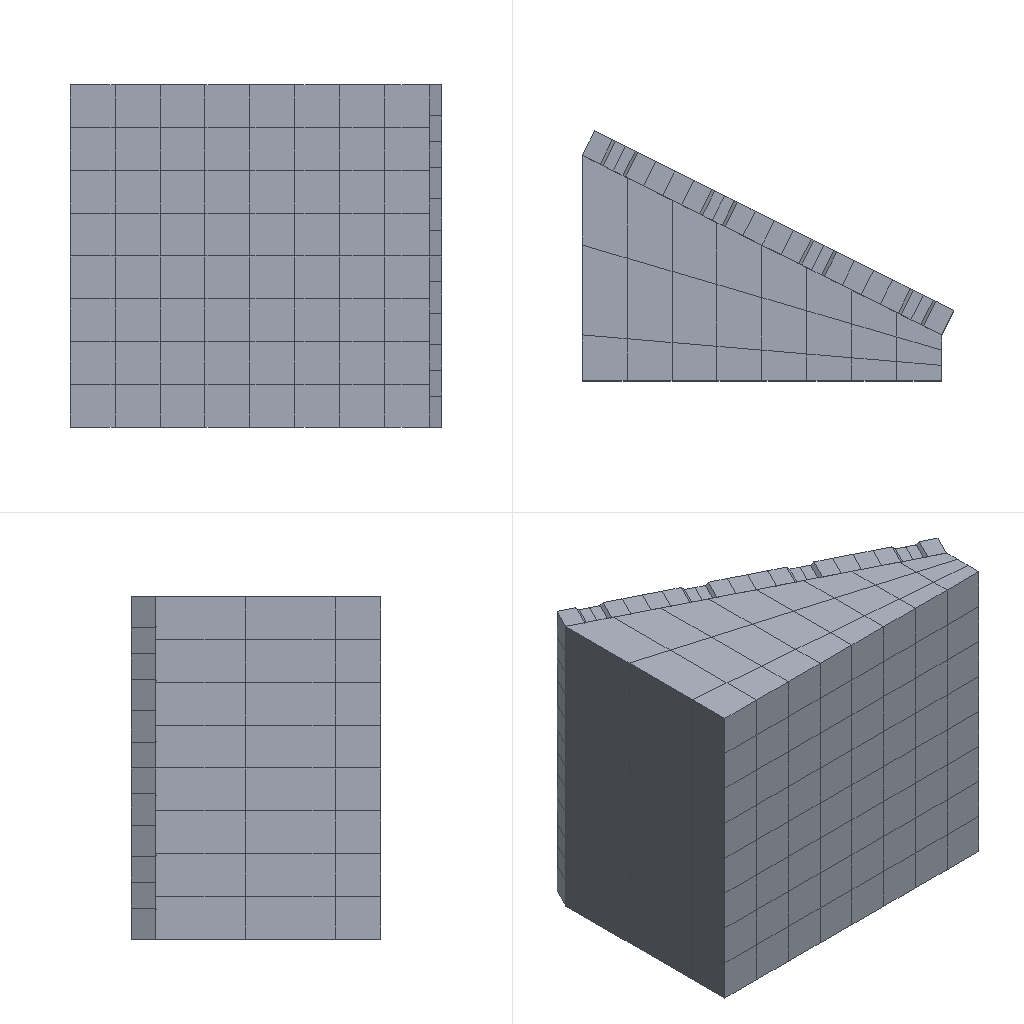Simulation study | abaqus
Set-up summary:
category,name,step,type,value,unit,region
solver,abaqus
solver,version,,,Abaqus/Standard 2020
units,not stated in the deck,,not stated
analysis,deck,,transient,transient
load_step,Step-2,Step-2,transient
load_step,requested,,,1
mesh,nodes,,,3205
mesh,elements,,,1224
element_type,C3D8R,,solid,1224
load,load commands in deck,,count,6
bc,support commands in deck,,count,8
material,HUNNINGTU,,in results
material,S,,in results
check,setup vs results,,match,"per instance, exact: element labels, types and connectivity; labels of the nodes the elements use; coordinates of those nodes at SINGLE_PRECISION in 15 of 31 instance(s)"
Abaqus input file, long lists of numbers shortened, first 402 of 1279 lines:
*Heading
** Job name: Job-1 Model name: Job-9
** Generated by: Abaqus/CAE 2020
*Preprint, echo=NO, model=NO, history=NO, contact=NO
**
** PARTS
**
*Part, name=BIKONGQIKUAI1
*Node
      1,  -23.409,         -15.,          12.
      2,  -23.409,  -10.17,          12.
** (128 more lines like these left out)
*Element, type=C3D8R
 1,  26,  33,  60,  27,  91,  98, 125,  92
 2,   1,   2,  44,  35,  66,  67, 109, 100
** (46 more lines like these left out)
*Nset, nset=SET-1, generate
   1,  130,    1
*Elset, elset=SET-1, generate
  1,  48,   1
** Section: Section-2-SET-1
*Solid Section, elset=SET-1, material=HUNNINGTU
,
*End Part
**
*Part, name=BIKONGQIKUAI1-COPY
*Node
      1,  0.1705,  -24.319,           0.
      2,  0.1705,  -5.681,           0.
** (62 more lines like these left out)
*Element, type=C3D8R
 1, 21,  3, 29, 25, 53, 35, 61, 57
 2, 22, 32, 30, 20, 54, 64, 62, 52
** (20 more lines like these left out)
*Nset, nset=SET-1, generate
  1,  64,   1
*Elset, elset=SET-1, generate
  1,  22,   1
** Section: Section-3-SET-1
*Solid Section, elset=SET-1, material=HUNNINGTU
,
*End Part
**
*Part, name=BIKONGQIKUAI1-COPY2
*Node
      1,   13.807,  -3.411,          12.
      2,   13.807,  -5.681,          12.
** (24 more lines like these left out)
*Element, type=C3D8R
1,  5, 18,  2,  1,  8, 24, 12, 13
2, 20,  3, 18,  5, 21, 23, 24,  8
** (4 more lines like these left out)
*Nset, nset=TIANCHONG, generate
  1,  26,   1
*Elset, elset=TIANCHONG, generate
 1,  6,  1
** Section: Section-4-TIANCHONG
*Solid Section, elset=TIANCHONG, material=HUNNINGTU
,
*End Part
**
*Part, name=PART-6
*Node
      1,  -157.419,   78.696,         150.
      2,  -137.741,   68.859,         150.
** (323 more lines like these left out)
*Element, type=C3D8R
  1,  82,  83,  92,  91,   1,   2,  11,  10
  2,  83,  84,  93,  92,   2,   3,  12,  11
** (190 more lines like these left out)
*Nset, nset=PART-6-REFPT_, internal
 325,
*Nset, nset=SET-2, generate
   1,  324,    1
*Elset, elset=SET-2, generate
   1,  192,    1
** Section: Section-1-SET-2
*Solid Section, elset=SET-2, material=S
,
*End Part
**
**
** ASSEMBLY
**
*Assembly, name=Assembly
**
*Instance, name=PART-6-1, part=PART-6
*End Instance
**
*Instance, name=BIKONGQIKUAI1-1, part=BIKONGQIKUAI1
-26.827, 13.414, 125.171
-26.827, 13.414, 125.171, -27.292, 14.167, 125.636, 106.047
*End Instance
**
*Instance, name=BIKONGQIKUAI1-COPY-1, part=BIKONGQIKUAI1-COPY
-48.579, 24.288, 150.171
-48.579, 24.288, 150.171, -49.045, 25.041, 150.636, 106.047
*End Instance
**
*Instance, name=BIKONGQIKUAI1-COPY2-1, part=BIKONGQIKUAI1-COPY2
-5.359, -10.734, 124.83
-5.359, -10.734, 124.83, -4.711, -10.333, 125.477, 223.65
*End Instance
**
*Instance, name=BIKONGQIKUAI1-1-LIN-1-2, part=BIKONGQIKUAI1
-26.827, 13.414, 75.171
-26.827, 13.414, 75.171, -27.292, 14.167, 75.636, 106.047
*End Instance
**
*Instance, name=BIKONGQIKUAI1-1-LIN-1-3, part=BIKONGQIKUAI1
-26.827, 13.414, 25.171
-26.827, 13.414, 25.171, -27.292, 14.167, 25.636, 106.047
*End Instance
**
*Instance, name=BIKONGQIKUAI1-1-LIN-2-1, part=BIKONGQIKUAI1
-48.579, 24.288, 100.17
-48.579, 24.288, 100.17, -49.045, 25.041, 100.635, 106.047
*End Instance
**
*Instance, name=BIKONGQIKUAI1-1-LIN-2-2, part=BIKONGQIKUAI1
-48.579, 24.288, 50.171
-48.579, 24.288, 50.171, -49.045, 25.041, 50.636, 106.047
*End Instance
**
*Instance, name=BIKONGQIKUAI1-1-LIN-2-3, part=BIKONGQIKUAI1
-70.331, 35.161, 25.17
-70.331, 35.161, 25.17, -70.797, 35.914, 25.635, 106.047
*End Instance
**
*Instance, name=BIKONGQIKUAI1-1-LIN-3-1, part=BIKONGQIKUAI1
-113.835, 56.909, 125.172
-113.835, 56.909, 125.172, -114.301, 57.662, 125.637, 106.047
*End Instance
**
*Instance, name=BIKONGQIKUAI1-1-LIN-3-2, part=BIKONGQIKUAI1
-92.083, 46.035, 100.171
-92.083, 46.035, 100.171, -92.549, 46.788, 100.636, 106.047
*End Instance
**
*Instance, name=BIKONGQIKUAI1-1-LIN-3-3, part=BIKONGQIKUAI1
-92.083, 46.035, 50.171
-92.083, 46.035, 50.171, -92.549, 46.788, 50.636, 106.047
*End Instance
**
*Instance, name=BIKONGQIKUAI1-1-LIN-4-1, part=BIKONGQIKUAI1
-113.835, 56.909, 75.17
-113.835, 56.909, 75.17, -114.301, 57.662, 75.635, 106.047
*End Instance
**
*Instance, name=BIKONGQIKUAI1-1-LIN-4-2, part=BIKONGQIKUAI1
-135.587, 67.782, 100.171
-135.587, 67.782, 100.171, -136.053, 68.535, 100.636, 106.047
*End Instance
**
*Instance, name=BIKONGQIKUAI1-1-LIN-4-3, part=BIKONGQIKUAI1
-157.34, 78.656, 125.172
-157.34, 78.656, 125.172, -157.805, 79.409, 125.637, 106.047
*End Instance
**
*Instance, name=BIKONGQIKUAI1-1-LIN-2-3-LIN-2-1, part=BIKONGQIKUAI1
-70.331, 35.161, 75.17
-70.331, 35.161, 75.17, -70.797, 35.914, 75.635, 106.047
*End Instance
**
*Instance, name=BIKONGQIKUAI1-1-LIN-2-3-LIN-3-1, part=BIKONGQIKUAI1
-70.331, 35.161, 125.17
-70.331, 35.161, 125.17, -70.797, 35.914, 125.635, 106.047
*End Instance
**
*Instance, name=BIKONGQIKUAI1-1-LIN-4-3-LIN-2-1, part=BIKONGQIKUAI1
-157.34, 78.656, 75.172
-157.34, 78.656, 75.172, -157.805, 79.409, 75.637, 106.047
*End Instance
**
*Instance, name=BIKONGQIKUAI1-1-LIN-4-3-LIN-3-1, part=BIKONGQIKUAI1
-157.34, 78.656, 25.172
-157.34, 78.656, 25.172, -157.805, 79.409, 25.637, 106.047
*End Instance
**
*Instance, name=BIKONGQIKUAI1-1-LIN-4-2-LIN-2-1, part=BIKONGQIKUAI1
-135.587, 67.782, 50.171
-135.587, 67.782, 50.171, -136.053, 68.535, 50.636, 106.047
*End Instance
**
*Instance, name=BIKONGQIKUAI1-1-LIN-4-2-LIN-3-1, part=BIKONGQIKUAI1
-113.835, 56.909, 25.17
-113.835, 56.909, 25.17, -114.301, 57.662, 25.635, 106.047
*End Instance
**
*Instance, name=BIKONGQIKUAI1-COPY-1-LIN-2-1, part=BIKONGQIKUAI1-COPY
-92.083, 46.035, 150.173
-92.083, 46.035, 150.173, -92.549, 46.788, 150.638, 106.047
*End Instance
**
*Instance, name=BIKONGQIKUAI1-COPY-1-LIN-3-1, part=BIKONGQIKUAI1-COPY
-135.587, 67.782, 150.173
-135.587, 67.782, 150.173, -136.053, 68.535, 150.638, 106.047
*End Instance
**
*Instance, name=BIKONGQIKUAI1-COPY-1-LIN-4-1, part=BIKONGQIKUAI1-COPY
-130.222, 78.516, -0.1725
-130.222, 78.516, -0.1725, -129.757, 77.763, 0.2929, 106.047
*End Instance
**
*Instance, name=BIKONGQIKUAI1-COPY-1-LIN-4-1-LIN-2-1, part=BIKONGQIKUAI1-COPY
-86.718, 56.769, -0.1725
-86.718, 56.769, -0.1725, -86.252, 56.016, 0.2929, 106.047
*End Instance
**
*Instance, name=BIKONGQIKUAI1-COPY-1-LIN-4-1-LIN-3-1, part=BIKONGQIKUAI1-COPY
-43.214, 35.021, -0.1715
-43.214, 35.021, -0.1715, -42.748, 34.268, 0.2939, 106.047
*End Instance
**
*Instance, name=BIKONGQIKUAI1-COPY2-1-LIN-2-1, part=BIKONGQIKUAI1-COPY2
-5.359, -10.734, 74.829
-5.359, -10.734, 74.829, -4.711, -10.333, 75.477, 223.65
*End Instance
**
*Instance, name=BIKONGQIKUAI1-COPY2-1-LIN-3-1, part=BIKONGQIKUAI1-COPY2
-5.359, -10.734, 24.829
-5.359, -10.734, 24.829, -4.711, -10.333, 25.477, 223.65
*End Instance
**
*Instance, name=BIKONGQIKUAI1-COPY2-1-LIN-3-1-LIN-2-1, part=BIKONGQIKUAI1-COPY2
-146.608, 100.123, 124.83
-146.608, 100.123, 124.83, -146.143, 99.37, 125.296, 106.047
*End Instance
**
*Instance, name=BIKONGQIKUAI1-COPY2-1-LIN-3--LIN-2-1, part=BIKONGQIKUAI1-COPY2
-146.608, 100.123, 74.831
-146.608, 100.123, 74.831, -146.143, 99.37, 75.296, 106.047
*End Instance
**
*Instance, name=BIKONGQIKUAI1-COPY2-1-LIN-3--LIN-3-1, part=BIKONGQIKUAI1-COPY2
-146.608, 100.123, 24.831
-146.608, 100.123, 24.831, -146.143, 99.37, 25.296, 106.047
*End Instance
**
*Nset, nset=DIMIAN, instance=PART-6-1, generate
 244,  324,    1
*Elset, elset=DIMIAN, instance=PART-6-1, generate
 129,  192,    1
*Nset, nset=SET-5, instance=BIKONGQIKUAI1-1
  4,  5, 30, 31, 69, 70, 95, 96
*Nset, nset=SET-5, instance=BIKONGQIKUAI1-1-LIN-1-3
 14, 15, 19, 20, 79, 80, 84, 85
*Nset, nset=SET-5, instance=BIKONGQIKUAI1-COPY-1-LIN-4-1-LIN-2-1
  1,  2, 18, 33, 34, 50
*Nset, nset=SET-5, instance=BIKONGQIKUAI1-1-LIN-2-3
 14, 15, 19, 20, 79, 80, 84, 85
*Nset, nset=SET-5, instance=BIKONGQIKUAI1-1-LIN-2-3-LIN-3-1
  4,  5, 30, 31, 69, 70, 95, 96
*Nset, nset=SET-5, instance=BIKONGQIKUAI1-1-LIN-4-2-LIN-3-1
 14, 15, 19, 20, 79, 80, 84, 85
*Nset, nset=SET-5, instance=BIKONGQIKUAI1-1-LIN-4-3
  4,  5, 30, 31, 69, 70, 95, 96
*Nset, nset=SET-5, instance=BIKONGQIKUAI1-1-LIN-4-3-LIN-3-1
 14, 15, 19, 20, 79, 80, 84, 85
*Nset, nset=SET-5, instance=BIKONGQIKUAI1-COPY-1
  1,  2, 18, 33, 34, 50
*Nset, nset=SET-5, instance=BIKONGQIKUAI1-COPY-1-LIN-3-1
  1,  2, 18, 33, 34, 50
*Nset, nset=SET-5, instance=BIKONGQIKUAI1-1-LIN-3-1
  4,  5, 30, 31, 69, 70, 95, 96
*Nset, nset=SET-5, instance=BIKONGQIKUAI1-COPY-1-LIN-2-1
  1,  2, 18, 33, 34, 50
*Nset, nset=SET-5, instance=BIKONGQIKUAI1-COPY-1-LIN-4-1-LIN-3-1
  1,  2, 18, 33, 34, 50
*Nset, nset=SET-5, instance=BIKONGQIKUAI1-COPY-1-LIN-4-1
  1,  2, 18, 33, 34, 50
*Elset, elset=SET-5, instance=BIKONGQIKUAI1-1
  4, 23
*Elset, elset=SET-5, instance=BIKONGQIKUAI1-1-LIN-1-3
 13, 20
*Elset, elset=SET-5, instance=BIKONGQIKUAI1-COPY-1-LIN-4-1-LIN-2-1
 17, 20
*Elset, elset=SET-5, instance=BIKONGQIKUAI1-1-LIN-2-3
 13, 20
*Elset, elset=SET-5, instance=BIKONGQIKUAI1-1-LIN-2-3-LIN-3-1
  4, 23
*Elset, elset=SET-5, instance=BIKONGQIKUAI1-1-LIN-4-2-LIN-3-1
 13, 20
*Elset, elset=SET-5, instance=BIKONGQIKUAI1-1-LIN-4-3
  4, 23
*Elset, elset=SET-5, instance=BIKONGQIKUAI1-1-LIN-4-3-LIN-3-1
 13, 20
*Elset, elset=SET-5, instance=BIKONGQIKUAI1-COPY-1
 17, 20
*Elset, elset=SET-5, instance=BIKONGQIKUAI1-COPY-1-LIN-3-1
 17, 20
*Elset, elset=SET-5, instance=BIKONGQIKUAI1-1-LIN-3-1
  4, 23
*Elset, elset=SET-5, instance=BIKONGQIKUAI1-COPY-1-LIN-2-1
 17, 20
*Elset, elset=SET-5, instance=BIKONGQIKUAI1-COPY-1-LIN-4-1-LIN-3-1
 17, 20
*Elset, elset=SET-5, instance=BIKONGQIKUAI1-COPY-1-LIN-4-1
 17, 20
*Nset, nset=SET-6, instance=BIKONGQIKUAI1-1
  6, 13, 71, 78
*Nset, nset=SET-6, instance=BIKONGQIKUAI1-1-LIN-1-2
  5,  6, 13, 14, 70, 71, 78, 79
*Nset, nset=SET-6, instance=BIKONGQIKUAI1-1-LIN-1-3
  6, 13, 71, 78
*Nset, nset=Set-97, instance=BIKONGQIKUAI1-1-LIN-1-3
 14, 15, 19, 20, 79, 80, 84, 85
*Nset, nset=Set-97, instance=BIKONGQIKUAI1-COPY-1-LIN-4-1-LIN-3-1
  1,  2, 18, 33, 34, 50
*Nset, nset=Set-97, instance=BIKONGQIKUAI1-1-LIN-2-3
 14, 15, 19, 20, 79, 80, 84, 85
*Nset, nset=Set-97, instance=BIKONGQIKUAI1-COPY-1-LIN-4-1-LIN-2-1
  1,  2, 18, 33, 34, 50
*Nset, nset=Set-97, instance=BIKONGQIKUAI1-1-LIN-2-3-LIN-3-1
  4,  5, 30, 31, 69, 70, 95, 96
*Nset, nset=Set-97, instance=BIKONGQIKUAI1-1-LIN-4-2-LIN-3-1
 14, 15, 19, 20, 79, 80, 84, 85
*Nset, nset=Set-97, instance=BIKONGQIKUAI1-1-LIN-4-3-LIN-3-1
 14, 15, 19, 20, 79, 80, 84, 85
*Nset, nset=Set-97, instance=BIKONGQIKUAI1-COPY-1
  1,  2, 18, 33, 34, 50
*Nset, nset=Set-97, instance=BIKONGQIKUAI1-1-LIN-4-3
  4,  5, 30, 31, 69, 70, 95, 96
*Nset, nset=Set-97, instance=BIKONGQIKUAI1-COPY-1-LIN-3-1
  1,  2, 18, 33, 34, 50
*Nset, nset=Set-97, instance=BIKONGQIKUAI1-COPY-1-LIN-4-1
  1,  2, 18, 33, 34, 50
*Nset, nset=Set-97, instance=BIKONGQIKUAI1-1-LIN-3-1
  4,  5, 30, 31, 69, 70, 95, 96
*Nset, nset=Set-97, instance=BIKONGQIKUAI1-1
  4,  5, 30, 31, 69, 70, 95, 96
*Nset, nset=Set-97, instance=BIKONGQIKUAI1-COPY-1-LIN-2-1
  1,  2, 18, 33, 34, 50
*Nset, nset=Set-98, instance=BIKONGQIKUAI1-1-LIN-1-3
  5,  6, 13, 14, 70, 71, 78, 79
*Nset, nset=Set-98, instance=BIKONGQIKUAI1-COPY2-1-LIN-3-1
 14, 15, 16, 17, 25, 26
*Nset, nset=Set-98, instance=BIKONGQIKUAI1-1-LIN-1-2
  5,  6, 13, 14, 70, 71, 78, 79
*Nset, nset=Set-98, instance=BIKONGQIKUAI1-COPY2-1-LIN-2-1
 14, 15, 16, 17, 25, 26
*Nset, nset=Set-98, instance=BIKONGQIKUAI1-1
  5,  6, 13, 14, 70, 71, 78, 79
*Nset, nset=Set-98, instance=BIKONGQIKUAI1-COPY2-1
 14, 15, 16, 17, 25, 26
*Nset, nset=Set-99, instance=BIKONGQIKUAI1-1-LIN-1-3
  5,  6, 13, 14, 70, 71, 78, 79
*Nset, nset=Set-99, instance=BIKONGQIKUAI1-COPY2-1-LIN-3-1
 14, 15, 16, 17, 25, 26
*Nset, nset=Set-99, instance=BIKONGQIKUAI1-1-LIN-1-2
  5,  6, 13, 14, 70, 71, 78, 79
*Nset, nset=Set-99, instance=BIKONGQIKUAI1-COPY2-1-LIN-3-1-LIN-2-1
 14, 15, 16, 17, 25, 26
*Nset, nset=Set-99, instance=BIKONGQIKUAI1-COPY2-1-LIN-2-1
 14, 15, 16, 17, 25, 26
*Nset, nset=Set-99, instance=BIKONGQIKUAI1-1-LIN-4-3-LIN-3-1
 20, 21, 29, 30, 85, 86, 94, 95
*Nset, nset=Set-99, instance=BIKONGQIKUAI1-1-LIN-4-3
 29, 30, 94, 95
*Nset, nset=Set-99, instance=BIKONGQIKUAI1-COPY2-1-LIN-3--LIN-3-1
 14, 15, 16, 17, 25, 26
*Nset, nset=Set-99, instance=BIKONGQIKUAI1-1
  5,  6, 13, 14, 70, 71, 78, 79
*Nset, nset=Set-99, instance=BIKONGQIKUAI1-COPY2-1-LIN-3--LIN-2-1
 14, 15, 16, 17, 25, 26
*Nset, nset=Set-99, instance=BIKONGQIKUAI1-1-LIN-4-3-LIN-2-1
 29, 30, 94, 95
*Nset, nset=Set-99, instance=BIKONGQIKUAI1-COPY2-1
 14, 15, 16, 17, 25, 26
*Elset, elset=_POMIAN_S2, internal, instance=PART-6-1, generate
  1,  64,   1
*Elset, elset=_SURF-3_S2, internal, instance=BIKONGQIKUAI1-1-LIN-3-2, generate
  1,  48,   1
*Elset, elset=_SURF-3_S2, internal, instance=BIKONGQIKUAI1-1-LIN-3-3, generate
  1,  48,   1
*Elset, elset=_SURF-3_S2, internal, instance=BIKONGQIKUAI1-1-LIN-4-1, generate
  1,  48,   1
*Elset, elset=_SURF-4_S2, internal, instance=BIKONGQIKUAI1-1-LIN-2-3-LIN-2-1, generate
  1,  48,   1
*Elset, elset=_SURF-5_S2, internal, instance=BIKONGQIKUAI1-1-LIN-3-2, generate
  1,  48,   1
*Elset, elset=_SURF-5_S2, internal, instance=BIKONGQIKUAI1-1-LIN-3-3, generate
  1,  48,   1
*Elset, elset=_SURF-5_S2, internal, instance=BIKONGQIKUAI1-1-LIN-4-1, generate
  1,  48,   1
*Elset, elset=_SURF-5_S2, internal, instance=BIKONGQIKUAI1-1-LIN-2-3-LIN-2-1, generate
  1,  48,   1
*Nset, nset="_T-Datum csys-2", internal, instance=BIKONGQIKUAI1-1
  6, 13, 71, 78
*Nset, nset="_T-Datum csys-2", internal, instance=BIKONGQIKUAI1-1-LIN-1-2
  5,  6, 13, 14, 70, 71, 78, 79
*Nset, nset="_T-Datum csys-2", internal, instance=BIKONGQIKUAI1-1-LIN-1-3
  6, 13, 71, 78
*Elset, elset=_ZHUANDIMIAN_S1, internal, instance=BIKONGQIKUAI1-COPY-1-LIN-2-1, generate
  1,  22,   1
*Elset, elset=_ZHUANDIMIAN_S1, internal, instance=BIKONGQIKUAI1-COPY2-1-LIN-2-1, generate
 1,  4,  1
*Elset, elset=_ZHUANDIMIAN_S1, internal, instance=BIKONGQIKUAI1-COPY-1-LIN-3-1, generate
  1,  22,   1
*Elset, elset=_ZHUANDIMIAN_S1, internal, instance=BIKONGQIKUAI1-COPY-1, generate
  1,  22,   1
*Elset, elset=_ZHUANDIMIAN_S1, internal, instance=BIKONGQIKUAI1-COPY2-1-LIN-3-1, generate
Last 655 lines:
 11,
*Elset, elset=__INT-2_GCS0_641_S4, internal, instance=BIKONGQIKUAI1-COPY-1-LIN-4-1-LIN-2-1
 14,
*Elset, elset=__INT-2_GCS0_648_S5, internal, instance=BIKONGQIKUAI1-COPY-1-LIN-4-1-LIN-2-1
 11,
*Elset, elset=__INT-2_GCS0_659_S4, internal, instance=BIKONGQIKUAI1-COPY-1-LIN-4-1-LIN-3-1
 14,
*Elset, elset=__INT-2_GCS0_666_S5, internal, instance=BIKONGQIKUAI1-COPY-1-LIN-4-1-LIN-3-1
 11,
*Surface, type=ELEMENT, name=POMIAN
_POMIAN_S2, S2
*Surface, type=ELEMENT, name=SURF-3
_SURF-3_S2, S2
*Surface, type=ELEMENT, name=SURF-4
_SURF-4_S2, S2
*Surface, type=ELEMENT, name=SURF-5
_SURF-5_S2, S2
*Elset, elset=_Surf-90_S1, internal, instance=BIKONGQIKUAI1-1-LIN-2-2, generate
  1,  48,   1
*Elset, elset=_Surf-90_S1, internal, instance=BIKONGQIKUAI1-1-LIN-1-3, generate
  1,  48,   1
*Elset, elset=_Surf-90_S1, internal, instance=BIKONGQIKUAI1-1-LIN-2-3, generate
  1,  48,   1
*Elset, elset=_Surf-90_S1, internal, instance=BIKONGQIKUAI1-1-LIN-2-3-LIN-3-1, generate
  1,  48,   1
*Elset, elset=_Surf-90_S1, internal, instance=BIKONGQIKUAI1-COPY-1-LIN-4-1-LIN-2-1, generate
  1,  22,   1
*Elset, elset=_Surf-90_S1, internal, instance=BIKONGQIKUAI1-1-LIN-1-2, generate
  1,  48,   1
*Elset, elset=_Surf-90_S1, internal, instance=BIKONGQIKUAI1-1-LIN-4-2-LIN-3-1, generate
  1,  48,   1
*Elset, elset=_Surf-90_S1, internal, instance=BIKONGQIKUAI1-1-LIN-4-1, generate
  1,  48,   1
*Elset, elset=_Surf-90_S1, internal, instance=BIKONGQIKUAI1-COPY2-1-LIN-3-1-LIN-2-1, generate
 1,  4,  1
*Elset, elset=_Surf-90_S1, internal, instance=BIKONGQIKUAI1-1-LIN-2-1, generate
  1,  48,   1
*Elset, elset=_Surf-90_S1, internal, instance=BIKONGQIKUAI1-1-LIN-3-2, generate
  1,  48,   1
*Elset, elset=_Surf-90_S1, internal, instance=BIKONGQIKUAI1-1-LIN-4-3-LIN-3-1, generate
  1,  48,   1
*Elset, elset=_Surf-90_S1, internal, instance=BIKONGQIKUAI1-1-LIN-4-3, generate
  1,  48,   1
*Elset, elset=_Surf-90_S1, internal, instance=BIKONGQIKUAI1-COPY2-1-LIN-3--LIN-3-1, generate
 1,  4,  1
*Elset, elset=_Surf-90_S1, internal, instance=BIKONGQIKUAI1-COPY-1-LIN-4-1-LIN-3-1, generate
  1,  22,   1
*Elset, elset=_Surf-90_S1, internal, instance=BIKONGQIKUAI1-1, generate
  1,  48,   1
*Elset, elset=_Surf-90_S1, internal, instance=BIKONGQIKUAI1-1-LIN-3-1, generate
  1,  48,   1
*Elset, elset=_Surf-90_S1, internal, instance=BIKONGQIKUAI1-1-LIN-4-3-LIN-2-1, generate
  1,  48,   1
*Elset, elset=_Surf-90_S1, internal, instance=BIKONGQIKUAI1-1-LIN-4-2, generate
  1,  48,   1
*Elset, elset=_Surf-90_S1, internal, instance=BIKONGQIKUAI1-COPY2-1-LIN-3--LIN-2-1, generate
 1,  4,  1
*Elset, elset=_Surf-90_S1, internal, instance=BIKONGQIKUAI1-1-LIN-3-3, generate
  1,  48,   1
*Elset, elset=_Surf-90_S1, internal, instance=BIKONGQIKUAI1-1-LIN-4-2-LIN-2-1, generate
  1,  48,   1
*Elset, elset=_Surf-90_S1, internal, instance=BIKONGQIKUAI1-1-LIN-2-3-LIN-2-1, generate
  1,  48,   1
*Elset, elset=_Surf-90_S1, internal, instance=BIKONGQIKUAI1-COPY-1-LIN-4-1, generate
  1,  22,   1
*Elset, elset=_Surf-90_S5, internal, instance=BIKONGQIKUAI1-COPY2-1-LIN-3-1-LIN-2-1
 5, 6
*Elset, elset=_Surf-90_S5, internal, instance=BIKONGQIKUAI1-COPY2-1-LIN-3--LIN-3-1
 5, 6
*Elset, elset=_Surf-90_S5, internal, instance=BIKONGQIKUAI1-COPY2-1-LIN-3--LIN-2-1
 5, 6
*Elset, elset=_Surf-90_S2, internal, instance=BIKONGQIKUAI1-COPY-1, generate
  1,  22,   1
*Elset, elset=_Surf-90_S2, internal, instance=BIKONGQIKUAI1-COPY2-1-LIN-2-1, generate
 1,  4,  1
*Elset, elset=_Surf-90_S2, internal, instance=BIKONGQIKUAI1-COPY-1-LIN-3-1, generate
  1,  22,   1
*Elset, elset=_Surf-90_S2, internal, instance=BIKONGQIKUAI1-COPY-1-LIN-2-1, generate
  1,  22,   1
*Elset, elset=_Surf-90_S2, internal, instance=BIKONGQIKUAI1-COPY2-1, generate
 1,  4,  1
*Elset, elset=_Surf-90_S2, internal, instance=BIKONGQIKUAI1-COPY2-1-LIN-3-1, generate
 1,  4,  1
*Elset, elset=_Surf-90_S3, internal, instance=BIKONGQIKUAI1-COPY2-1-LIN-2-1
 5, 6
*Elset, elset=_Surf-90_S3, internal, instance=BIKONGQIKUAI1-COPY2-1
 5, 6
*Elset, elset=_Surf-90_S3, internal, instance=BIKONGQIKUAI1-COPY2-1-LIN-3-1
 5, 6
*Surface, type=ELEMENT, name=Surf-90
_Surf-90_S1, S1
_Surf-90_S5, S5
_Surf-90_S2, S2
_Surf-90_S3, S3
*Elset, elset=_Surf-91_S1, internal, instance=BIKONGQIKUAI1-1-LIN-2-2
  1,  2,  3,  4,  5,  6,  7,  8,  9, 10, 11, 12, 15, 16, 18, 19
 20, 21, 22, 24, 25, 26, 27, 28, 29, 30, 31, 32, 33, 34, 35, 36
** (1 more lines like these left out)
*Elset, elset=_Surf-91_S1, internal, instance=BIKONGQIKUAI1-1-LIN-1-3, generate
  1,  48,   1
*Elset, elset=_Surf-91_S1, internal, instance=BIKONGQIKUAI1-1-LIN-2-1
  1,  2,  3,  4,  5,  6,  7,  8,  9, 10, 11, 12, 15, 16, 18, 19
 20, 21, 22, 24, 25, 26, 27, 28, 29, 30, 31, 32, 33, 34, 35, 36
** (1 more lines like these left out)
*Elset, elset=_Surf-91_S1, internal, instance=BIKONGQIKUAI1-1-LIN-1-2, generate
  1,  48,   1
*Elset, elset=_Surf-91_S1, internal, instance=BIKONGQIKUAI1-COPY-1-LIN-4-1-LIN-3-1
  1,  2,  3,  4,  6,  7,  8,  9, 10, 11, 12, 13, 14, 15, 16, 17
 18, 19, 20, 22
*Elset, elset=_Surf-91_S1, internal, instance=BIKONGQIKUAI1-1, generate
  1,  48,   1
*Elset, elset=_Surf-91_S2, internal, instance=BIKONGQIKUAI1-COPY-1
  1,  2,  3,  4,  6,  7,  8,  9, 10, 11, 12, 13, 14, 15, 16, 17
 18, 19, 20, 22
*Elset, elset=_Surf-91_S2, internal, instance=BIKONGQIKUAI1-COPY2-1-LIN-2-1, generate
 1,  4,  1
*Elset, elset=_Surf-91_S2, internal, instance=BIKONGQIKUAI1-COPY2-1-LIN-3-1, generate
 1,  4,  1
*Elset, elset=_Surf-91_S2, internal, instance=BIKONGQIKUAI1-COPY2-1, generate
 1,  4,  1
*Elset, elset=_Surf-91_S3, internal, instance=BIKONGQIKUAI1-COPY2-1-LIN-2-1
 5, 6
*Elset, elset=_Surf-91_S3, internal, instance=BIKONGQIKUAI1-COPY2-1-LIN-3-1
 5, 6
*Elset, elset=_Surf-91_S3, internal, instance=BIKONGQIKUAI1-COPY2-1
 5, 6
*Surface, type=ELEMENT, name=Surf-91
_Surf-91_S1, S1
_Surf-91_S2, S2
_Surf-91_S3, S3
*Elset, elset=_Surf-92_S1, internal, instance=BIKONGQIKUAI1-1-LIN-2-2
  1, 13, 14, 15, 17, 22, 23, 24, 25, 27, 29, 34, 35, 36, 41
*Elset, elset=_Surf-92_S1, internal, instance=BIKONGQIKUAI1-COPY-1-LIN-4-1-LIN-3-1
  1,  5, 10, 11, 16, 21
*Elset, elset=_Surf-92_S1, internal, instance=BIKONGQIKUAI1-1-LIN-2-3, generate
  1,  48,   1
*Elset, elset=_Surf-92_S1, internal, instance=BIKONGQIKUAI1-1-LIN-2-3-LIN-3-1, generate
  1,  48,   1
*Elset, elset=_Surf-92_S1, internal, instance=BIKONGQIKUAI1-COPY-1-LIN-4-1-LIN-2-1
  2,  3,  4,  6,  7,  8,  9, 12, 13, 14, 15, 17, 19, 22
*Elset, elset=_Surf-92_S1, internal, instance=BIKONGQIKUAI1-1-LIN-2-1
  1, 13, 14, 15, 17, 22, 23, 24, 25, 27, 29, 34, 35, 36, 41
*Elset, elset=_Surf-92_S1, internal, instance=BIKONGQIKUAI1-1-LIN-3-2
  2,  3,  4,  5,  6,  7,  8,  9, 10, 11, 12, 16, 18, 19, 20, 21
 26, 28, 30, 31, 32, 33, 35, 37, 38, 39, 40, 43, 44, 45, 46, 47
*Elset, elset=_Surf-92_S1, internal, instance=BIKONGQIKUAI1-1-LIN-3-3
  2,  3,  4,  5,  6,  7,  8,  9, 10, 11, 12, 16, 18, 19, 20, 21
 26, 28, 30, 31, 32, 33, 35, 37, 38, 39, 40, 43, 44, 45, 46, 47
*Elset, elset=_Surf-92_S1, internal, instance=BIKONGQIKUAI1-1-LIN-2-3-LIN-2-1, generate
  1,  48,   1
*Elset, elset=_Surf-92_S2, internal, instance=BIKONGQIKUAI1-COPY-1
  1,  5, 10, 11, 16, 21
*Elset, elset=_Surf-92_S2, internal, instance=BIKONGQIKUAI1-COPY-1-LIN-2-1
  2,  3,  4,  6,  7,  8,  9, 12, 13, 14, 15, 17, 19, 22
*Surface, type=ELEMENT, name=Surf-92
_Surf-92_S1, S1
_Surf-92_S2, S2
*Elset, elset=_Surf-93_S1, internal, instance=BIKONGQIKUAI1-1-LIN-3-3
  1,  2, 11, 12, 13, 14, 15, 17, 22, 23, 24, 25, 27, 29, 30, 34
 35, 36, 41, 48
*Elset, elset=_Surf-93_S1, internal, instance=BIKONGQIKUAI1-COPY-1-LIN-4-1-LIN-2-1
  1,  5,  6,  7, 10, 11, 16, 18, 20, 21
*Elset, elset=_Surf-93_S1, internal, instance=BIKONGQIKUAI1-1-LIN-4-2-LIN-3-1, generate
  1,  48,   1
*Elset, elset=_Surf-93_S1, internal, instance=BIKONGQIKUAI1-1-LIN-4-1, generate
  1,  48,   1
*Elset, elset=_Surf-93_S1, internal, instance=BIKONGQIKUAI1-1-LIN-3-2
  1,  2, 11, 12, 13, 14, 15, 17, 22, 23, 24, 25, 27, 29, 30, 34
 35, 36, 41, 48
*Elset, elset=_Surf-93_S1, internal, instance=BIKONGQIKUAI1-1-LIN-3-1, generate
  1,  48,   1
*Elset, elset=_Surf-93_S1, internal, instance=BIKONGQIKUAI1-1-LIN-4-2
  3,  4,  5,  6,  7,  8,  9, 10, 16, 18, 19, 20, 21, 26, 31, 32
 33, 37, 40, 43, 44, 45, 46
*Elset, elset=_Surf-93_S1, internal, instance=BIKONGQIKUAI1-1-LIN-4-2-LIN-2-1
  3,  4,  5,  6,  7,  8,  9, 10, 16, 18, 19, 20, 21, 26, 31, 32
 33, 37, 40, 43, 44, 45, 46
*Elset, elset=_Surf-93_S1, internal, instance=BIKONGQIKUAI1-COPY-1-LIN-4-1
  2,  3,  4,  8,  9, 12, 13, 14, 15, 17, 19, 22
*Elset, elset=_Surf-93_S2, internal, instance=BIKONGQIKUAI1-COPY-1-LIN-3-1
  2,  3,  4,  8,  9, 12, 13, 14, 15, 17, 19, 22
*Elset, elset=_Surf-93_S2, internal, instance=BIKONGQIKUAI1-COPY-1-LIN-2-1
  1,  5,  6,  7, 10, 11, 16, 18, 20, 21
*Surface, type=ELEMENT, name=Surf-93
_Surf-93_S1, S1
_Surf-93_S2, S2
*Elset, elset=_Surf-94_S1, internal, instance=BIKONGQIKUAI1-1-LIN-4-2
  1,  2, 11, 12, 13, 14, 15, 17, 22, 23, 24, 25, 27, 28, 29, 30
 34, 35, 36, 38, 41, 42, 46, 47, 48
*Elset, elset=_Surf-94_S1, internal, instance=BIKONGQIKUAI1-1-LIN-4-3, generate
  1,  48,   1
*Elset, elset=_Surf-94_S1, internal, instance=BIKONGQIKUAI1-1-LIN-4-3-LIN-3-1, generate
  1,  48,   1
*Elset, elset=_Surf-94_S1, internal, instance=BIKONGQIKUAI1-COPY2-1-LIN-3-1-LIN-2-1, generate
 1,  4,  1
*Elset, elset=_Surf-94_S1, internal, instance=BIKONGQIKUAI1-COPY2-1-LIN-3--LIN-3-1, generate
 1,  4,  1
*Elset, elset=_Surf-94_S1, internal, instance=BIKONGQIKUAI1-1-LIN-4-3-LIN-2-1, generate
  1,  48,   1
*Elset, elset=_Surf-94_S1, internal, instance=BIKONGQIKUAI1-COPY2-1-LIN-3--LIN-2-1, generate
 1,  4,  1
*Elset, elset=_Surf-94_S1, internal, instance=BIKONGQIKUAI1-1-LIN-4-2-LIN-2-1
  1,  2, 11, 12, 13, 14, 15, 17, 22, 23, 24, 25, 27, 28, 29, 30
 34, 35, 36, 38, 41, 42, 46, 47, 48
*Elset, elset=_Surf-94_S1, internal, instance=BIKONGQIKUAI1-COPY-1-LIN-4-1
  1,  5,  6,  7, 10, 11, 16, 18, 20, 21
*Elset, elset=_Surf-94_S5, internal, instance=BIKONGQIKUAI1-COPY2-1-LIN-3-1-LIN-2-1
 5, 6
*Elset, elset=_Surf-94_S5, internal, instance=BIKONGQIKUAI1-COPY2-1-LIN-3--LIN-3-1
 5, 6
*Elset, elset=_Surf-94_S5, internal, instance=BIKONGQIKUAI1-COPY2-1-LIN-3--LIN-2-1
 5, 6
*Elset, elset=_Surf-94_S2, internal, instance=BIKONGQIKUAI1-COPY-1-LIN-3-1
  1,  5,  6,  7, 10, 11, 16, 18, 20, 21
*Surface, type=ELEMENT, name=Surf-94
_Surf-94_S1, S1
_Surf-94_S5, S5
_Surf-94_S2, S2
*Elset, elset=_Surf-95_S1, internal, instance=BIKONGQIKUAI1-1-LIN-3-3
  1,  2, 14, 15, 17, 22, 23, 24, 25, 29, 30, 35, 36, 41, 48
*Elset, elset=_Surf-95_S1, internal, instance=BIKONGQIKUAI1-1-LIN-4-2-LIN-3-1
  1,  2,  3,  4,  5,  6, 15, 16, 17, 19, 23, 24, 28, 29, 30, 31
 32, 35, 37, 43, 45
*Elset, elset=_Surf-95_S1, internal, instance=BIKONGQIKUAI1-1-LIN-3-2
  1,  2, 11, 12, 13, 14, 15, 17, 22, 23, 24, 25, 27, 29, 30, 34
 35, 36, 41, 48
*Elset, elset=_Surf-95_S1, internal, instance=BIKONGQIKUAI1-1-LIN-4-1, generate
  1,  48,   1
*Elset, elset=_Surf-95_S1, internal, instance=BIKONGQIKUAI1-1-LIN-3-1
  7,  8,  9, 10, 11, 12, 13, 14, 18, 20, 21, 22, 26, 27, 33, 34
 36, 38, 40, 41, 46, 47, 48
*Elset, elset=_Surf-95_S1, internal, instance=BIKONGQIKUAI1-1-LIN-4-2
  3,  4,  5,  6,  7,  8,  9, 10, 16, 18, 19, 20, 21, 26, 31, 32
 33, 37, 40, 43, 44, 45, 46
*Elset, elset=_Surf-95_S1, internal, instance=BIKONGQIKUAI1-1-LIN-4-2-LIN-2-1
  3,  4,  5,  6,  8,  9, 10, 16, 18, 19, 26, 31, 32, 33, 37, 40
 43, 44, 45, 46
*Surface, type=ELEMENT, name=Surf-95
_Surf-95_S1, S1
*Elset, elset=_Surf-96_S1, internal, instance=BIKONGQIKUAI1-1-LIN-3-3
 17, 23
*Elset, elset=_Surf-96_S1, internal, instance=BIKONGQIKUAI1-1-LIN-3-2
 13, 14
*Elset, elset=_Surf-96_S1, internal, instance=BIKONGQIKUAI1-1-LIN-4-1
  1,  2,  3,  6,  7,  8,  9, 11, 12, 15, 16, 18, 19, 21, 22, 24
 25, 26, 27, 28, 29, 30, 31, 32, 33, 34, 35, 36, 37, 38, 39, 40
** (1 more lines like these left out)
*Elset, elset=_Surf-96_S1, internal, instance=BIKONGQIKUAI1-1-LIN-4-2
 10, 20
*Elset, elset=_Surf-96_S1, internal, instance=BIKONGQIKUAI1-1-LIN-4-2-LIN-2-1
 4, 5
*Surface, type=ELEMENT, name=Surf-96
_Surf-96_S1, S1
*Elset, elset=_Surf-97_S1, internal, instance=BIKONGQIKUAI1-1-LIN-4-1, generate
  1,  48,   1
*Surface, type=ELEMENT, name=Surf-97
_Surf-97_S1, S1
*Elset, elset=_Surf-98_S1, internal, instance=BIKONGQIKUAI1-1-LIN-3-1, generate
  1,  48,   1
*Surface, type=ELEMENT, name=Surf-98
_Surf-98_S1, S1
*Elset, elset=_Surf-99_S1, internal, instance=BIKONGQIKUAI1-1-LIN-4-2-LIN-3-1, generate
  1,  48,   1
*Surface, type=ELEMENT, name=Surf-99
_Surf-99_S1, S1
*Elset, elset=_Surf-100_S1, internal, instance=BIKONGQIKUAI1-1-LIN-4-2, generate
  1,  48,   1
*Surface, type=ELEMENT, name=Surf-100
_Surf-100_S1, S1
*Elset, elset=_Surf-101_S1, internal, instance=BIKONGQIKUAI1-1-LIN-4-2-LIN-2-1, generate
  1,  48,   1
*Surface, type=ELEMENT, name=Surf-101
_Surf-101_S1, S1
*Elset, elset=_Surf-102_S1, internal, instance=BIKONGQIKUAI1-1-LIN-3-2, generate
  1,  48,   1
*Surface, type=ELEMENT, name=Surf-102
_Surf-102_S1, S1
*Elset, elset=_Surf-103_S1, internal, instance=BIKONGQIKUAI1-1-LIN-3-3, generate
  1,  48,   1
*Surface, type=ELEMENT, name=Surf-103
_Surf-103_S1, S1
*Elset, elset=_ZHUANDIMIAN_S2_1, internal, instance=BIKONGQIKUAI1-1, generate
  1,  48,   1
*Elset, elset=_ZHUANDIMIAN_S2_1, internal, instance=BIKONGQIKUAI1-1-LIN-1-2, generate
  1,  48,   1
*Elset, elset=_ZHUANDIMIAN_S2_1, internal, instance=BIKONGQIKUAI1-1-LIN-3-2, generate
  1,  48,   1
*Elset, elset=_ZHUANDIMIAN_S2_1, internal, instance=BIKONGQIKUAI1-1-LIN-2-3, generate
  1,  48,   1
*Elset, elset=_ZHUANDIMIAN_S2_1, internal, instance=BIKONGQIKUAI1-COPY-1-LIN-4-1-LIN-2-1, generate
  1,  22,   1
*Elset, elset=_ZHUANDIMIAN_S2_1, internal, instance=BIKONGQIKUAI1-1-LIN-2-3-LIN-3-1, generate
  1,  48,   1
*Elset, elset=_ZHUANDIMIAN_S2_1, internal, instance=BIKONGQIKUAI1-1-LIN-4-1, generate
  1,  48,   1
*Elset, elset=_ZHUANDIMIAN_S2_1, internal, instance=BIKONGQIKUAI1-1-LIN-4-2-LIN-3-1, generate
  1,  48,   1
*Elset, elset=_ZHUANDIMIAN_S2_1, internal, instance=BIKONGQIKUAI1-COPY2-1-LIN-3-1-LIN-2-1, generate
 1,  4,  1
*Elset, elset=_ZHUANDIMIAN_S2_1, internal, instance=BIKONGQIKUAI1-1-LIN-2-1, generate
  1,  48,   1
*Elset, elset=_ZHUANDIMIAN_S2_1, internal, instance=BIKONGQIKUAI1-1-LIN-4-3-LIN-3-1, generate
  1,  48,   1
*Elset, elset=_ZHUANDIMIAN_S2_1, internal, instance=BIKONGQIKUAI1-1-LIN-4-3, generate
  1,  48,   1
*Elset, elset=_ZHUANDIMIAN_S2_1, internal, instance=BIKONGQIKUAI1-COPY2-1-LIN-3--LIN-3-1, generate
 1,  4,  1
*Elset, elset=_ZHUANDIMIAN_S2_1, internal, instance=BIKONGQIKUAI1-1-LIN-2-2, generate
  1,  48,   1
*Elset, elset=_ZHUANDIMIAN_S2_1, internal, instance=BIKONGQIKUAI1-1-LIN-4-2, generate
  1,  48,   1
*Elset, elset=_ZHUANDIMIAN_S2_1, internal, instance=BIKONGQIKUAI1-1-LIN-4-3-LIN-2-1, generate
  1,  48,   1
*Elset, elset=_ZHUANDIMIAN_S2_1, internal, instance=BIKONGQIKUAI1-1-LIN-3-1, generate
  1,  48,   1
*Elset, elset=_ZHUANDIMIAN_S2_1, internal, instance=BIKONGQIKUAI1-COPY-1-LIN-4-1-LIN-3-1, generate
  1,  22,   1
*Elset, elset=_ZHUANDIMIAN_S2_1, internal, instance=BIKONGQIKUAI1-1-LIN-1-3, generate
  1,  48,   1
*Elset, elset=_ZHUANDIMIAN_S2_1, internal, instance=BIKONGQIKUAI1-COPY2-1-LIN-3--LIN-2-1, generate
 1,  4,  1
*Elset, elset=_ZHUANDIMIAN_S2_1, internal, instance=BIKONGQIKUAI1-1-LIN-2-3-LIN-2-1, generate
  1,  48,   1
*Elset, elset=_ZHUANDIMIAN_S2_1, internal, instance=BIKONGQIKUAI1-1-LIN-4-2-LIN-2-1, generate
  1,  48,   1
*Elset, elset=_ZHUANDIMIAN_S2_1, internal, instance=BIKONGQIKUAI1-1-LIN-3-3, generate
  1,  48,   1
*Elset, elset=_ZHUANDIMIAN_S2_1, internal, instance=BIKONGQIKUAI1-COPY-1-LIN-4-1, generate
  1,  22,   1
*Elset, elset=_ZHUANDIMIAN_S3_1, internal, instance=BIKONGQIKUAI1-COPY2-1-LIN-3-1-LIN-2-1
 5, 6
*Elset, elset=_ZHUANDIMIAN_S3_1, internal, instance=BIKONGQIKUAI1-COPY2-1-LIN-3--LIN-3-1
 5, 6
*Elset, elset=_ZHUANDIMIAN_S3_1, internal, instance=BIKONGQIKUAI1-COPY2-1-LIN-3--LIN-2-1
 5, 6
*Elset, elset=_ZHUANDIMIAN_S1_1, internal, instance=BIKONGQIKUAI1-COPY2-1-LIN-2-1, generate
 1,  4,  1
*Elset, elset=_ZHUANDIMIAN_S1_1, internal, instance=BIKONGQIKUAI1-COPY-1, generate
  1,  22,   1
*Elset, elset=_ZHUANDIMIAN_S1_1, internal, instance=BIKONGQIKUAI1-COPY-1-LIN-3-1, generate
  1,  22,   1
*Elset, elset=_ZHUANDIMIAN_S1_1, internal, instance=BIKONGQIKUAI1-COPY-1-LIN-2-1, generate
  1,  22,   1
*Elset, elset=_ZHUANDIMIAN_S1_1, internal, instance=BIKONGQIKUAI1-COPY2-1, generate
 1,  4,  1
*Elset, elset=_ZHUANDIMIAN_S1_1, internal, instance=BIKONGQIKUAI1-COPY2-1-LIN-3-1, generate
 1,  4,  1
*Elset, elset=_ZHUANDIMIAN_S5_1, internal, instance=BIKONGQIKUAI1-COPY2-1-LIN-2-1
 5, 6
*Elset, elset=_ZHUANDIMIAN_S5_1, internal, instance=BIKONGQIKUAI1-COPY2-1
 5, 6
*Elset, elset=_ZHUANDIMIAN_S5_1, internal, instance=BIKONGQIKUAI1-COPY2-1-LIN-3-1
 5, 6
*Surface, type=ELEMENT, name=ZHUANDIMIAN
_ZHUANDIMIAN_S2_1, S2
_ZHUANDIMIAN_S3_1, S3
_ZHUANDIMIAN_S1_1, S1
_ZHUANDIMIAN_S5_1, S5
*Surface, type=ELEMENT, name=_INT-2_GCS0_16, internal
__INT-2_GCS0_16_S5, S5
*Surface, type=ELEMENT, name=_INT-2_GCS0_17, internal
__INT-2_GCS0_17_S4, S4
*Surface, type=ELEMENT, name=_INT-2_GCS0_31, internal
__INT-2_GCS0_31_S4, S4
*Surface, type=ELEMENT, name=_INT-2_GCS0_33, internal
__INT-2_GCS0_33_S3, S3
*Surface, type=ELEMENT, name=_INT-2_GCS0_46, internal
__INT-2_GCS0_46_S4, S4
*Surface, type=ELEMENT, name=_INT-2_GCS0_53, internal
__INT-2_GCS0_53_S5, S5
*Surface, type=ELEMENT, name=_INT-2_GCS0_77, internal
__INT-2_GCS0_77_S5, S5
*Surface, type=ELEMENT, name=_INT-2_GCS0_78, internal
__INT-2_GCS0_78_S4, S4
*Surface, type=ELEMENT, name=_INT-2_GCS0_92, internal
__INT-2_GCS0_92_S4, S4
*Surface, type=ELEMENT, name=_INT-2_GCS0_94, internal
__INT-2_GCS0_94_S3, S3
*Surface, type=ELEMENT, name=_INT-2_GCS0_107, internal
__INT-2_GCS0_107_S5, S5
*Surface, type=ELEMENT, name=_INT-2_GCS0_108, internal
__INT-2_GCS0_108_S4, S4
*Surface, type=ELEMENT, name=_INT-2_GCS0_122, internal
__INT-2_GCS0_122_S4, S4
*Surface, type=ELEMENT, name=_INT-2_GCS0_124, internal
__INT-2_GCS0_124_S3, S3
*Surface, type=ELEMENT, name=_INT-2_GCS0_137, internal
__INT-2_GCS0_137_S5, S5
*Surface, type=ELEMENT, name=_INT-2_GCS0_138, internal
__INT-2_GCS0_138_S4, S4
*Surface, type=ELEMENT, name=_INT-2_GCS0_152, internal
__INT-2_GCS0_152_S4, S4
*Surface, type=ELEMENT, name=_INT-2_GCS0_154, internal
__INT-2_GCS0_154_S3, S3
*Surface, type=ELEMENT, name=_INT-2_GCS0_167, internal
__INT-2_GCS0_167_S5, S5
*Surface, type=ELEMENT, name=_INT-2_GCS0_168, internal
__INT-2_GCS0_168_S4, S4
*Surface, type=ELEMENT, name=_INT-2_GCS0_182, internal
__INT-2_GCS0_182_S4, S4
*Surface, type=ELEMENT, name=_INT-2_GCS0_184, internal
__INT-2_GCS0_184_S3, S3
*Surface, type=ELEMENT, name=_INT-2_GCS0_197, internal
__INT-2_GCS0_197_S5, S5
*Surface, type=ELEMENT, name=_INT-2_GCS0_198, internal
__INT-2_GCS0_198_S4, S4
*Surface, type=ELEMENT, name=_INT-2_GCS0_212, internal
__INT-2_GCS0_212_S4, S4
*Surface, type=ELEMENT, name=_INT-2_GCS0_214, internal
__INT-2_GCS0_214_S3, S3
*Surface, type=ELEMENT, name=_INT-2_GCS0_227, internal
__INT-2_GCS0_227_S5, S5
*Surface, type=ELEMENT, name=_INT-2_GCS0_228, internal
__INT-2_GCS0_228_S4, S4
*Surface, type=ELEMENT, name=_INT-2_GCS0_242, internal
__INT-2_GCS0_242_S4, S4
*Surface, type=ELEMENT, name=_INT-2_GCS0_244, internal
__INT-2_GCS0_244_S3, S3
*Surface, type=ELEMENT, name=_INT-2_GCS0_257, internal
__INT-2_GCS0_257_S5, S5
*Surface, type=ELEMENT, name=_INT-2_GCS0_258, internal
__INT-2_GCS0_258_S4, S4
*Surface, type=ELEMENT, name=_INT-2_GCS0_272, internal
__INT-2_GCS0_272_S4, S4
*Surface, type=ELEMENT, name=_INT-2_GCS0_274, internal
__INT-2_GCS0_274_S3, S3
*Surface, type=ELEMENT, name=_INT-2_GCS0_287, internal
__INT-2_GCS0_287_S5, S5
*Surface, type=ELEMENT, name=_INT-2_GCS0_288, internal
__INT-2_GCS0_288_S4, S4
*Surface, type=ELEMENT, name=_INT-2_GCS0_302, internal
__INT-2_GCS0_302_S4, S4
*Surface, type=ELEMENT, name=_INT-2_GCS0_304, internal
__INT-2_GCS0_304_S3, S3
*Surface, type=ELEMENT, name=_INT-2_GCS0_317, internal
__INT-2_GCS0_317_S5, S5
*Surface, type=ELEMENT, name=_INT-2_GCS0_318, internal
__INT-2_GCS0_318_S4, S4
*Surface, type=ELEMENT, name=_INT-2_GCS0_332, internal
__INT-2_GCS0_332_S4, S4
*Surface, type=ELEMENT, name=_INT-2_GCS0_334, internal
__INT-2_GCS0_334_S3, S3
*Surface, type=ELEMENT, name=_INT-2_GCS0_347, internal
__INT-2_GCS0_347_S5, S5
*Surface, type=ELEMENT, name=_INT-2_GCS0_348, internal
__INT-2_GCS0_348_S4, S4
*Surface, type=ELEMENT, name=_INT-2_GCS0_362, internal
__INT-2_GCS0_362_S4, S4
*Surface, type=ELEMENT, name=_INT-2_GCS0_364, internal
__INT-2_GCS0_364_S3, S3
*Surface, type=ELEMENT, name=_INT-2_GCS0_377, internal
__INT-2_GCS0_377_S5, S5
*Surface, type=ELEMENT, name=_INT-2_GCS0_378, internal
__INT-2_GCS0_378_S4, S4
*Surface, type=ELEMENT, name=_INT-2_GCS0_392, internal
__INT-2_GCS0_392_S4, S4
*Surface, type=ELEMENT, name=_INT-2_GCS0_394, internal
__INT-2_GCS0_394_S3, S3
*Surface, type=ELEMENT, name=_INT-2_GCS0_407, internal
__INT-2_GCS0_407_S5, S5
*Surface, type=ELEMENT, name=_INT-2_GCS0_408, internal
__INT-2_GCS0_408_S4, S4
*Surface, type=ELEMENT, name=_INT-2_GCS0_422, internal
__INT-2_GCS0_422_S4, S4
*Surface, type=ELEMENT, name=_INT-2_GCS0_424, internal
__INT-2_GCS0_424_S3, S3
*Surface, type=ELEMENT, name=_INT-2_GCS0_437, internal
__INT-2_GCS0_437_S5, S5
*Surface, type=ELEMENT, name=_INT-2_GCS0_438, internal
__INT-2_GCS0_438_S4, S4
*Surface, type=ELEMENT, name=_INT-2_GCS0_452, internal
__INT-2_GCS0_452_S4, S4
*Surface, type=ELEMENT, name=_INT-2_GCS0_454, internal
__INT-2_GCS0_454_S3, S3
*Surface, type=ELEMENT, name=_INT-2_GCS0_467, internal
__INT-2_GCS0_467_S5, S5
*Surface, type=ELEMENT, name=_INT-2_GCS0_468, internal
__INT-2_GCS0_468_S4, S4
*Surface, type=ELEMENT, name=_INT-2_GCS0_482, internal
__INT-2_GCS0_482_S4, S4
*Surface, type=ELEMENT, name=_INT-2_GCS0_484, internal
__INT-2_GCS0_484_S3, S3
*Surface, type=ELEMENT, name=_INT-2_GCS0_497, internal
__INT-2_GCS0_497_S5, S5
*Surface, type=ELEMENT, name=_INT-2_GCS0_498, internal
__INT-2_GCS0_498_S4, S4
*Surface, type=ELEMENT, name=_INT-2_GCS0_512, internal
__INT-2_GCS0_512_S4, S4
*Surface, type=ELEMENT, name=_INT-2_GCS0_514, internal
__INT-2_GCS0_514_S3, S3
*Surface, type=ELEMENT, name=_INT-2_GCS0_527, internal
__INT-2_GCS0_527_S5, S5
*Surface, type=ELEMENT, name=_INT-2_GCS0_528, internal
__INT-2_GCS0_528_S4, S4
*Surface, type=ELEMENT, name=_INT-2_GCS0_542, internal
__INT-2_GCS0_542_S4, S4
*Surface, type=ELEMENT, name=_INT-2_GCS0_544, internal
__INT-2_GCS0_544_S3, S3
*Surface, type=ELEMENT, name=_INT-2_GCS0_557, internal
__INT-2_GCS0_557_S5, S5
*Surface, type=ELEMENT, name=_INT-2_GCS0_558, internal
__INT-2_GCS0_558_S4, S4
*Surface, type=ELEMENT, name=_INT-2_GCS0_572, internal
__INT-2_GCS0_572_S4, S4
*Surface, type=ELEMENT, name=_INT-2_GCS0_574, internal
__INT-2_GCS0_574_S3, S3
*Surface, type=ELEMENT, name=_INT-2_GCS0_587, internal
__INT-2_GCS0_587_S4, S4
*Surface, type=ELEMENT, name=_INT-2_GCS0_594, internal
__INT-2_GCS0_594_S5, S5
*Surface, type=ELEMENT, name=_INT-2_GCS0_605, internal
__INT-2_GCS0_605_S4, S4
*Surface, type=ELEMENT, name=_INT-2_GCS0_612, internal
__INT-2_GCS0_612_S5, S5
*Surface, type=ELEMENT, name=_INT-2_GCS0_623, internal
__INT-2_GCS0_623_S4, S4
*Surface, type=ELEMENT, name=_INT-2_GCS0_630, internal
__INT-2_GCS0_630_S5, S5
*Surface, type=ELEMENT, name=_INT-2_GCS0_641, internal
__INT-2_GCS0_641_S4, S4
*Surface, type=ELEMENT, name=_INT-2_GCS0_648, internal
__INT-2_GCS0_648_S5, S5
*Surface, type=ELEMENT, name=_INT-2_GCS0_659, internal
__INT-2_GCS0_659_S4, S4
*Surface, type=ELEMENT, name=_INT-2_GCS0_666, internal
__INT-2_GCS0_666_S5, S5
*End Assembly
*Amplitude, name=AMP-1, definition=PERIODIC
1,             24.,              0.,              0.
             1.,              0.
*Amplitude, name=Amp-2
             0.,              0.,              1.,              1.
**
** MATERIALS
**
*Material, name=HUNNINGTU
*Density
 2.4e-05,
*Elastic
 3e+06, 0.3
*Material, name=S
*Density
 3e-05,
*Elastic
 3e+07, 0.22
**
** INTERACTION PROPERTIES
**
*Surface Interaction, name=INTPROP-1
1.,
*Friction, slip tolerance=0.005
 0.35,
*Surface Behavior, pressure-overclosure=HARD
*Surface Interaction, name=INTPROP-2
1.,
*Friction, slip tolerance=0.005
 0.4,
*Surface Behavior, pressure-overclosure=HARD
**
** BOUNDARY CONDITIONS
**
** Name: BC-8 Type: 对称/反对称/完全固定
*Boundary
Set-99, ENCASTRE
** Name: Disp-BC-1 Type: 位移/转角
*Boundary
DIMIAN, 1, 1
** Name: Disp-BC-2 Type: 位移/转角
*Boundary
DIMIAN, 2, 2
** Name: Disp-BC-3 Type: 位移/转角
*Boundary
DIMIAN, 3, 3
** Name: Disp-BC-4 Type: 位移/转角
*Boundary
DIMIAN, 4, 4
** Name: Disp-BC-5 Type: 位移/转角
*Boundary
DIMIAN, 5, 5
** Name: Disp-BC-6 Type: 位移/转角
*Boundary
DIMIAN, 6, 6
** Name: Disp-BC-7 Type: 位移/转角
*Boundary
Set-97, 3, 3
**
** INTERACTIONS
**
** Interaction: INTPROP-1-1
*Contact Pair, interaction=INTPROP-1, type=SURFACE TO SURFACE
ZHUANDIMIAN, POMIAN
** Interaction: general_contact
*Contact
*Contact Inclusions, ALL EXTERIOR
*Contact Property Assignment
 ,  , INTPROP-2
** ----------------------------------------------------------------
**
** STEP: Step-2
**
*Step, name=Step-2, nlgeom=YES, inc=1000
*Dynamic
0.01,1.,1e-05
**
** LOADS
**
** Name: Load-1-Copy2   Type: Surface traction
*Dsload, amplitude=Amp-2
Surf-97, TRVEC, 2.5, 0.4471, 0.8945, -2.36849e-08
** Name: Load-1-Copy2-Copy3   Type: Surface traction
*Dsload, amplitude=Amp-2
Surf-100, TRVEC, 1., 0.4471, 0.8945, -2.36849e-08
** Name: Load-1-Copy2-Copy4   Type: Surface traction
*Dsload, amplitude=Amp-2
Surf-101, TRVEC, 1., 0.4471, 0.8945, -2.36849e-08
** Name: Load-1-Copy2-Copy5   Type: Surface traction
*Dsload, amplitude=Amp-2
Surf-102, TRVEC, 1., 0.4471, 0.8945, -2.36849e-08
** Name: Load-1-Copy2-Copy6   Type: Surface traction
*Dsload, amplitude=Amp-2
Surf-103, TRVEC, 1., 0.4471, 0.8945, -2.36849e-08
** Name: Load-5   Type: Gravity
*Dload
, GRAV, 980., 0., -1., 0.
**
** OUTPUT REQUESTS
**
*Restart, write, frequency=0
**
** FIELD OUTPUT: F-Output-3
**
*Output, field, frequency=5
*Contact Output
CDISP, CSTRESS
**
** FIELD OUTPUT: F-Output-1
**
*Node Output
CF, RF, RT, U, V
**
** FIELD OUTPUT: F-Output-2
**
*Element Output, directions=YES
E, LE, MISES, MISESMAX, P, PE, PEEQ, PEEQMAX, PEMAG, S, SF, VEEQ
**
** HISTORY OUTPUT: H-Output-2
**
*Output, history
*Contact Output
CDISP, CSTRESS
**
** HISTORY OUTPUT: H-Output-1
**
*Output, history, variable=PRESELECT
*End Step
Results summary:
result,step,,completed,increments=20 time=1.0/1.0
result,analysis,,,transient
result,last_loadstep,,,1
result,primary field,,,U
result,reaction total,,FX,-3314.859,model units
result,reaction total,,FY,41821.189,model units
result,reaction total,,FZ,0.6395,model units